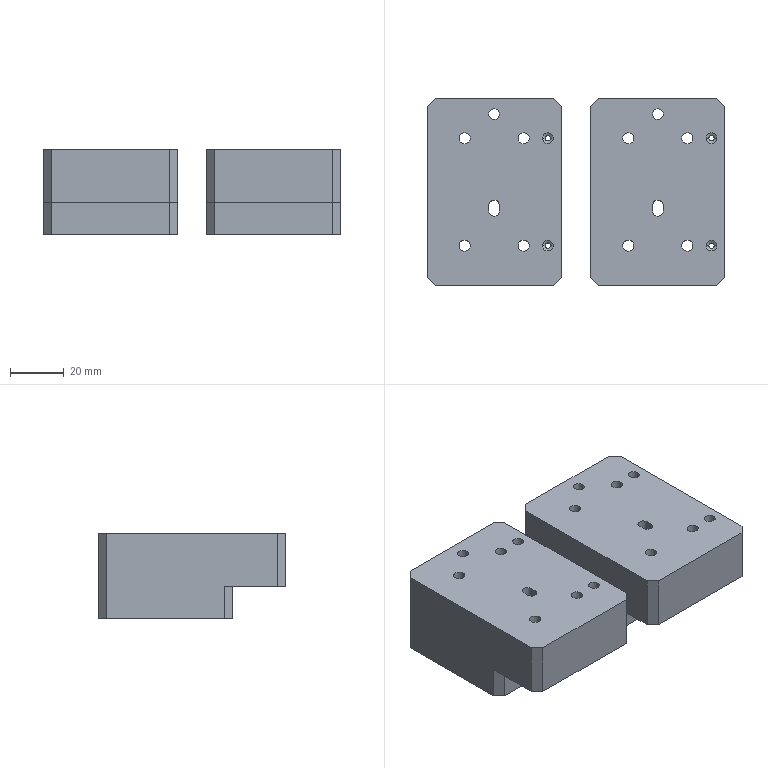NC program | NX | posted with a generic post | part box 111 x 70 x 32 mm
Lines 19 to 875 of 5357:
(ZLEVEL_PROFILE , TOOL : D10)
N36 T15 M6
N38 G54
N40 G17 G0 G90 X104.574 Y75.1 S9500 M3
N42 G43 Z30. H15
N44 Z1.5
N46 G94 G1 X108.554 Z1.291 F1000.
N48 X109.963 Y74.74 Z1.215
N50 X111.215 Y73.998 Z1.139
N52 X114.998 Y70.215 Z0.859
N54 X115.74 Y68.963 Z0.782
N56 X116.1 Y67.554 Z0.706
N58 Y35. Z-1.
N60 Y3. F3000.
N62 G2 X114.606 Y-0.606 R5.1
N64 G1 X111.606 Y-3.606
N66 G2 X108. Y-5.1 R5.1
N68 G1 X64.
N70 G2 X60.394 Y-3.606 R5.1
N72 G1 X57.394 Y-0.606
N74 G2 X55.9 Y3. R5.1
N76 G1 Y67.
N78 G2 X57.394 Y70.606 R5.1
N80 G1 X60.394 Y73.606
N82 G2 X64. Y75.1 R5.1
N84 G1 X108.
N86 G2 X111.606 Y73.606 R5.1
N88 G1 X114.606 Y70.606
N90 G2 X116.1 Y67. R5.1
N92 G1 Y35.
N94 Y3. Z-1.121
N96 X116.075 Y2.5 Z-1.123
N98 X116.002 Y2.005 Z-1.125
N100 X115.88 Y1.52 Z-1.126
N102 X115.712 Y1.048 Z-1.128
N104 X115.498 Y0.596 Z-1.13
N106 X115.24 Y0.167 Z-1.132
N108 X114.942 Y-0.235 Z-1.134
N110 X114.606 Y-0.606 Z-1.136
N112 X111.606 Y-3.606 Z-1.152
N114 X111.235 Y-3.942 Z-1.154
N116 X110.833 Y-4.24 Z-1.156
N118 X110.404 Y-4.498 Z-1.158
N120 X109.952 Y-4.712 Z-1.159
N122 X109.48 Y-4.88 Z-1.161
N124 X108.995 Y-5.002 Z-1.163
N126 X108.5 Y-5.075 Z-1.165
N128 X108. Y-5.1 Z-1.167
N130 X64. Z-1.333
N132 X63.5 Y-5.075 Z-1.335
N134 X63.005 Y-5.002 Z-1.337
N136 X62.52 Y-4.88 Z-1.339
N138 X62.048 Y-4.712 Z-1.341
N140 X61.596 Y-4.498 Z-1.342
N142 X61.167 Y-4.24 Z-1.344
N144 X60.765 Y-3.942 Z-1.346
N146 X60.394 Y-3.606 Z-1.348
N148 X57.394 Y-0.606 Z-1.364
N150 X57.058 Y-0.235 Z-1.366
N152 X56.76 Y0.167 Z-1.368
N154 X56.502 Y0.596 Z-1.37
N156 X56.288 Y1.048 Z-1.372
N158 X56.12 Y1.52 Z-1.374
N160 X55.998 Y2.005 Z-1.375
N162 X55.925 Y2.5 Z-1.377
N164 X55.9 Y3. Z-1.379
N166 Y67. Z-1.621
N168 X55.925 Y67.5 Z-1.623
N170 X55.998 Y67.995 Z-1.625
N172 X56.12 Y68.48 Z-1.626
N174 X56.288 Y68.952 Z-1.628
N176 X56.502 Y69.404 Z-1.63
N178 X56.76 Y69.833 Z-1.632
N180 X57.058 Y70.235 Z-1.634
N182 X57.394 Y70.606 Z-1.636
N184 X60.394 Y73.606 Z-1.652
N186 X60.765 Y73.942 Z-1.654
N188 X61.167 Y74.24 Z-1.656
N190 X61.596 Y74.498 Z-1.658
N192 X62.048 Y74.712 Z-1.659
N194 X62.52 Y74.88 Z-1.661
N196 X63.005 Y75.002 Z-1.663
N198 X63.5 Y75.075 Z-1.665
N200 X64. Y75.1 Z-1.667
N202 X108. Z-1.833
N204 X108.5 Y75.075 Z-1.835
N206 X108.995 Y75.002 Z-1.837
N208 X109.48 Y74.88 Z-1.839
N210 X109.952 Y74.712 Z-1.841
N212 X110.404 Y74.498 Z-1.842
N214 X110.833 Y74.24 Z-1.844
N216 X111.235 Y73.942 Z-1.846
N218 X111.606 Y73.606 Z-1.848
N220 X114.606 Y70.606 Z-1.864
N222 X114.942 Y70.235 Z-1.866
N224 X115.24 Y69.833 Z-1.868
N226 X115.498 Y69.404 Z-1.87
N228 X115.712 Y68.952 Z-1.872
N230 X115.88 Y68.48 Z-1.874
N232 X116.002 Y67.995 Z-1.875
N234 X116.075 Y67.5 Z-1.877
N236 X116.1 Y67. Z-1.879
N238 Y35. Z-2.
N240 Y3. Z-2.121
N242 X116.075 Y2.5 Z-2.123
N244 X116.002 Y2.005 Z-2.125
N246 X115.88 Y1.52 Z-2.126
N248 X115.712 Y1.048 Z-2.128
N250 X115.498 Y0.596 Z-2.13
N252 X115.24 Y0.167 Z-2.132
N254 X114.942 Y-0.235 Z-2.134
N256 X114.606 Y-0.606 Z-2.136
N258 X111.606 Y-3.606 Z-2.152
N260 X111.235 Y-3.942 Z-2.154
N262 X110.833 Y-4.24 Z-2.156
N264 X110.404 Y-4.498 Z-2.158
N266 X109.952 Y-4.712 Z-2.159
N268 X109.48 Y-4.88 Z-2.161
N270 X108.995 Y-5.002 Z-2.163
N272 X108.5 Y-5.075 Z-2.165
N274 X108. Y-5.1 Z-2.167
N276 X64. Z-2.333
N278 X63.5 Y-5.075 Z-2.335
N280 X63.005 Y-5.002 Z-2.337
N282 X62.52 Y-4.88 Z-2.339
N284 X62.048 Y-4.712 Z-2.341
N286 X61.596 Y-4.498 Z-2.342
N288 X61.167 Y-4.24 Z-2.344
N290 X60.765 Y-3.942 Z-2.346
N292 X60.394 Y-3.606 Z-2.348
N294 X57.394 Y-0.606 Z-2.364
N296 X57.058 Y-0.235 Z-2.366
N298 X56.76 Y0.167 Z-2.368
N300 X56.502 Y0.596 Z-2.37
N302 X56.288 Y1.048 Z-2.372
N304 X56.12 Y1.52 Z-2.374
N306 X55.998 Y2.005 Z-2.375
N308 X55.925 Y2.5 Z-2.377
N310 X55.9 Y3. Z-2.379
N312 Y67. Z-2.621
N314 X55.925 Y67.5 Z-2.623
N316 X55.998 Y67.995 Z-2.625
N318 X56.12 Y68.48 Z-2.626
N320 X56.288 Y68.952 Z-2.628
N322 X56.502 Y69.404 Z-2.63
N324 X56.76 Y69.833 Z-2.632
N326 X57.058 Y70.235 Z-2.634
N328 X57.394 Y70.606 Z-2.636
N330 X60.394 Y73.606 Z-2.652
N332 X60.765 Y73.942 Z-2.654
N334 X61.167 Y74.24 Z-2.656
N336 X61.596 Y74.498 Z-2.658
N338 X62.048 Y74.712 Z-2.659
N340 X62.52 Y74.88 Z-2.661
N342 X63.005 Y75.002 Z-2.663
N344 X63.5 Y75.075 Z-2.665
N346 X64. Y75.1 Z-2.667
N348 X108. Z-2.833
N350 X108.5 Y75.075 Z-2.835
N352 X108.995 Y75.002 Z-2.837
N354 X109.48 Y74.88 Z-2.839
N356 X109.952 Y74.712 Z-2.841
N358 X110.404 Y74.498 Z-2.842
N360 X110.833 Y74.24 Z-2.844
N362 X111.235 Y73.942 Z-2.846
N364 X111.606 Y73.606 Z-2.848
N366 X114.606 Y70.606 Z-2.864
N368 X114.942 Y70.235 Z-2.866
N370 X115.24 Y69.833 Z-2.868
N372 X115.498 Y69.404 Z-2.87
N374 X115.712 Y68.952 Z-2.872
N376 X115.88 Y68.48 Z-2.874
N378 X116.002 Y67.995 Z-2.875
N380 X116.075 Y67.5 Z-2.877
N382 X116.1 Y67. Z-2.879
N384 Y35. Z-3.
N386 Y3. Z-3.121
N388 X116.075 Y2.5 Z-3.123
N390 X116.002 Y2.005 Z-3.125
N392 X115.88 Y1.52 Z-3.126
N394 X115.712 Y1.048 Z-3.128
N396 X115.498 Y0.596 Z-3.13
N398 X115.24 Y0.167 Z-3.132
N400 X114.942 Y-0.235 Z-3.134
N402 X114.606 Y-0.606 Z-3.136
N404 X111.606 Y-3.606 Z-3.152
N406 X111.235 Y-3.942 Z-3.154
N408 X110.833 Y-4.24 Z-3.156
N410 X110.404 Y-4.498 Z-3.158
N412 X109.952 Y-4.712 Z-3.159
N414 X109.48 Y-4.88 Z-3.161
N416 X108.995 Y-5.002 Z-3.163
N418 X108.5 Y-5.075 Z-3.165
N420 X108. Y-5.1 Z-3.167
N422 X64. Z-3.333
N424 X63.5 Y-5.075 Z-3.335
N426 X63.005 Y-5.002 Z-3.337
N428 X62.52 Y-4.88 Z-3.339
N430 X62.048 Y-4.712 Z-3.341
N432 X61.596 Y-4.498 Z-3.342
N434 X61.167 Y-4.24 Z-3.344
N436 X60.765 Y-3.942 Z-3.346
N438 X60.394 Y-3.606 Z-3.348
N440 X57.394 Y-0.606 Z-3.364
N442 X57.058 Y-0.235 Z-3.366
N444 X56.76 Y0.167 Z-3.368
N446 X56.502 Y0.596 Z-3.37
N448 X56.288 Y1.048 Z-3.372
N450 X56.12 Y1.52 Z-3.374
N452 X55.998 Y2.005 Z-3.375
N454 X55.925 Y2.5 Z-3.377
N456 X55.9 Y3. Z-3.379
N458 Y67. Z-3.621
N460 X55.925 Y67.5 Z-3.623
N462 X55.998 Y67.995 Z-3.625
N464 X56.12 Y68.48 Z-3.626
N466 X56.288 Y68.952 Z-3.628
N468 X56.502 Y69.404 Z-3.63
N470 X56.76 Y69.833 Z-3.632
N472 X57.058 Y70.235 Z-3.634
N474 X57.394 Y70.606 Z-3.636
N476 X60.394 Y73.606 Z-3.652
N478 X60.765 Y73.942 Z-3.654
N480 X61.167 Y74.24 Z-3.656
N482 X61.596 Y74.498 Z-3.658
N484 X62.048 Y74.712 Z-3.659
N486 X62.52 Y74.88 Z-3.661
N488 X63.005 Y75.002 Z-3.663
N490 X63.5 Y75.075 Z-3.665
N492 X64. Y75.1 Z-3.667
N494 X108. Z-3.833
N496 X108.5 Y75.075 Z-3.835
N498 X108.995 Y75.002 Z-3.837
N500 X109.48 Y74.88 Z-3.839
N502 X109.952 Y74.712 Z-3.841
N504 X110.404 Y74.498 Z-3.842
N506 X110.833 Y74.24 Z-3.844
N508 X111.235 Y73.942 Z-3.846
N510 X111.606 Y73.606 Z-3.848
N512 X114.606 Y70.606 Z-3.864
N514 X114.942 Y70.235 Z-3.866
N516 X115.24 Y69.833 Z-3.868
N518 X115.498 Y69.404 Z-3.87
N520 X115.712 Y68.952 Z-3.872
N522 X115.88 Y68.48 Z-3.874
N524 X116.002 Y67.995 Z-3.875
N526 X116.075 Y67.5 Z-3.877
N528 X116.1 Y67. Z-3.879
N530 Y35. Z-4.
N532 Y3. Z-4.121
N534 X116.075 Y2.5 Z-4.123
N536 X116.002 Y2.005 Z-4.125
N538 X115.88 Y1.52 Z-4.126
N540 X115.712 Y1.048 Z-4.128
N542 X115.498 Y0.596 Z-4.13
N544 X115.24 Y0.167 Z-4.132
N546 X114.942 Y-0.235 Z-4.134
N548 X114.606 Y-0.606 Z-4.136
N550 X111.606 Y-3.606 Z-4.152
N552 X111.235 Y-3.942 Z-4.154
N554 X110.833 Y-4.24 Z-4.156
N556 X110.404 Y-4.498 Z-4.158
N558 X109.952 Y-4.712 Z-4.159
N560 X109.48 Y-4.88 Z-4.161
N562 X108.995 Y-5.002 Z-4.163
N564 X108.5 Y-5.075 Z-4.165
N566 X108. Y-5.1 Z-4.167
N568 X64. Z-4.333
N570 X63.5 Y-5.075 Z-4.335
N572 X63.005 Y-5.002 Z-4.337
N574 X62.52 Y-4.88 Z-4.339
N576 X62.048 Y-4.712 Z-4.341
N578 X61.596 Y-4.498 Z-4.342
N580 X61.167 Y-4.24 Z-4.344
N582 X60.765 Y-3.942 Z-4.346
N584 X60.394 Y-3.606 Z-4.348
N586 X57.394 Y-0.606 Z-4.364
N588 X57.058 Y-0.235 Z-4.366
N590 X56.76 Y0.167 Z-4.368
N592 X56.502 Y0.596 Z-4.37
N594 X56.288 Y1.048 Z-4.372
N596 X56.12 Y1.52 Z-4.374
N598 X55.998 Y2.005 Z-4.375
N600 X55.925 Y2.5 Z-4.377
N602 X55.9 Y3. Z-4.379
N604 Y67. Z-4.621
N606 X55.925 Y67.5 Z-4.623
N608 X55.998 Y67.995 Z-4.625
N610 X56.12 Y68.48 Z-4.626
N612 X56.288 Y68.952 Z-4.628
N614 X56.502 Y69.404 Z-4.63
N616 X56.76 Y69.833 Z-4.632
N618 X57.058 Y70.235 Z-4.634
N620 X57.394 Y70.606 Z-4.636
N622 X60.394 Y73.606 Z-4.652
N624 X60.765 Y73.942 Z-4.654
N626 X61.167 Y74.24 Z-4.656
N628 X61.596 Y74.498 Z-4.658
N630 X62.048 Y74.712 Z-4.659
N632 X62.52 Y74.88 Z-4.661
N634 X63.005 Y75.002 Z-4.663
N636 X63.5 Y75.075 Z-4.665
N638 X64. Y75.1 Z-4.667
N640 X108. Z-4.833
N642 X108.5 Y75.075 Z-4.835
N644 X108.995 Y75.002 Z-4.837
N646 X109.48 Y74.88 Z-4.839
N648 X109.952 Y74.712 Z-4.841
N650 X110.404 Y74.498 Z-4.842
N652 X110.833 Y74.24 Z-4.844
N654 X111.235 Y73.942 Z-4.846
N656 X111.606 Y73.606 Z-4.848
N658 X114.606 Y70.606 Z-4.864
N660 X114.942 Y70.235 Z-4.866
N662 X115.24 Y69.833 Z-4.868
N664 X115.498 Y69.404 Z-4.87
N666 X115.712 Y68.952 Z-4.872
N668 X115.88 Y68.48 Z-4.874
N670 X116.002 Y67.995 Z-4.875
N672 X116.075 Y67.5 Z-4.877
N674 X116.1 Y67. Z-4.879
N676 Y35. Z-5.
N678 Y3. Z-5.121
N680 X116.075 Y2.5 Z-5.123
N682 X116.002 Y2.005 Z-5.125
N684 X115.88 Y1.52 Z-5.126
N686 X115.712 Y1.048 Z-5.128
N688 X115.498 Y0.596 Z-5.13
N690 X115.24 Y0.167 Z-5.132
N692 X114.942 Y-0.235 Z-5.134
N694 X114.606 Y-0.606 Z-5.136
N696 X111.606 Y-3.606 Z-5.152
N698 X111.235 Y-3.942 Z-5.154
N700 X110.833 Y-4.24 Z-5.156
N702 X110.404 Y-4.498 Z-5.158
N704 X109.952 Y-4.712 Z-5.159
N706 X109.48 Y-4.88 Z-5.161
N708 X108.995 Y-5.002 Z-5.163
N710 X108.5 Y-5.075 Z-5.165
N712 X108. Y-5.1 Z-5.167
N714 X64. Z-5.333
N716 X63.5 Y-5.075 Z-5.335
N718 X63.005 Y-5.002 Z-5.337
N720 X62.52 Y-4.88 Z-5.339
N722 X62.048 Y-4.712 Z-5.341
N724 X61.596 Y-4.498 Z-5.342
N726 X61.167 Y-4.24 Z-5.344
N728 X60.765 Y-3.942 Z-5.346
N730 X60.394 Y-3.606 Z-5.348
N732 X57.394 Y-0.606 Z-5.364
N734 X57.058 Y-0.235 Z-5.366
N736 X56.76 Y0.167 Z-5.368
N738 X56.502 Y0.596 Z-5.37
N740 X56.288 Y1.048 Z-5.372
N742 X56.12 Y1.52 Z-5.374
N744 X55.998 Y2.005 Z-5.375
N746 X55.925 Y2.5 Z-5.377
N748 X55.9 Y3. Z-5.379
N750 Y67. Z-5.621
N752 X55.925 Y67.5 Z-5.623
N754 X55.998 Y67.995 Z-5.625
N756 X56.12 Y68.48 Z-5.626
N758 X56.288 Y68.952 Z-5.628
N760 X56.502 Y69.404 Z-5.63
N762 X56.76 Y69.833 Z-5.632
N764 X57.058 Y70.235 Z-5.634
N766 X57.394 Y70.606 Z-5.636
N768 X60.394 Y73.606 Z-5.652
N770 X60.765 Y73.942 Z-5.654
N772 X61.167 Y74.24 Z-5.656
N774 X61.596 Y74.498 Z-5.658
N776 X62.048 Y74.712 Z-5.659
N778 X62.52 Y74.88 Z-5.661
N780 X63.005 Y75.002 Z-5.663
N782 X63.5 Y75.075 Z-5.665
N784 X64. Y75.1 Z-5.667
N786 X108. Z-5.833
N788 X108.5 Y75.075 Z-5.835
N790 X108.995 Y75.002 Z-5.837
N792 X109.48 Y74.88 Z-5.839
N794 X109.952 Y74.712 Z-5.841
N796 X110.404 Y74.498 Z-5.842
N798 X110.833 Y74.24 Z-5.844
N800 X111.235 Y73.942 Z-5.846
N802 X111.606 Y73.606 Z-5.848
N804 X114.606 Y70.606 Z-5.864
N806 X114.942 Y70.235 Z-5.866
N808 X115.24 Y69.833 Z-5.868
N810 X115.498 Y69.404 Z-5.87
N812 X115.712 Y68.952 Z-5.872
N814 X115.88 Y68.48 Z-5.874
N816 X116.002 Y67.995 Z-5.875
N818 X116.075 Y67.5 Z-5.877
N820 X116.1 Y67. Z-5.879
N822 Y35. Z-6.
N824 Y3. Z-6.121
N826 X116.075 Y2.5 Z-6.123
N828 X116.002 Y2.005 Z-6.125
N830 X115.88 Y1.52 Z-6.126
N832 X115.712 Y1.048 Z-6.128
N834 X115.498 Y0.596 Z-6.13
N836 X115.24 Y0.167 Z-6.132
N838 X114.942 Y-0.235 Z-6.134
N840 X114.606 Y-0.606 Z-6.136
N842 X111.606 Y-3.606 Z-6.152
N844 X111.235 Y-3.942 Z-6.154
N846 X110.833 Y-4.24 Z-6.156
N848 X110.404 Y-4.498 Z-6.158
N850 X109.952 Y-4.712 Z-6.159
N852 X109.48 Y-4.88 Z-6.161
N854 X108.995 Y-5.002 Z-6.163
N856 X108.5 Y-5.075 Z-6.165
N858 X108. Y-5.1 Z-6.167
N860 X64. Z-6.333
N862 X63.5 Y-5.075 Z-6.335
N864 X63.005 Y-5.002 Z-6.337
N866 X62.52 Y-4.88 Z-6.339
N868 X62.048 Y-4.712 Z-6.341
N870 X61.596 Y-4.498 Z-6.342
N872 X61.167 Y-4.24 Z-6.344
N874 X60.765 Y-3.942 Z-6.346
N876 X60.394 Y-3.606 Z-6.348
N878 X57.394 Y-0.606 Z-6.364
N880 X57.058 Y-0.235 Z-6.366
N882 X56.76 Y0.167 Z-6.368
N884 X56.502 Y0.596 Z-6.37
N886 X56.288 Y1.048 Z-6.372
N888 X56.12 Y1.52 Z-6.374
N890 X55.998 Y2.005 Z-6.375
N892 X55.925 Y2.5 Z-6.377
N894 X55.9 Y3. Z-6.379
N896 Y67. Z-6.621
N898 X55.925 Y67.5 Z-6.623
N900 X55.998 Y67.995 Z-6.625
N902 X56.12 Y68.48 Z-6.626
N904 X56.288 Y68.952 Z-6.628
N906 X56.502 Y69.404 Z-6.63
N908 X56.76 Y69.833 Z-6.632
N910 X57.058 Y70.235 Z-6.634
N912 X57.394 Y70.606 Z-6.636
N914 X60.394 Y73.606 Z-6.652
N916 X60.765 Y73.942 Z-6.654
N918 X61.167 Y74.24 Z-6.656
N920 X61.596 Y74.498 Z-6.658
N922 X62.048 Y74.712 Z-6.659
N924 X62.52 Y74.88 Z-6.661
N926 X63.005 Y75.002 Z-6.663
N928 X63.5 Y75.075 Z-6.665
N930 X64. Y75.1 Z-6.667
N932 X108. Z-6.833
N934 X108.5 Y75.075 Z-6.835
N936 X108.995 Y75.002 Z-6.837
N938 X109.48 Y74.88 Z-6.839
N940 X109.952 Y74.712 Z-6.841
N942 X110.404 Y74.498 Z-6.842
N944 X110.833 Y74.24 Z-6.844
N946 X111.235 Y73.942 Z-6.846
N948 X111.606 Y73.606 Z-6.848
N950 X114.606 Y70.606 Z-6.864
N952 X114.942 Y70.235 Z-6.866
N954 X115.24 Y69.833 Z-6.868
N956 X115.498 Y69.404 Z-6.87
N958 X115.712 Y68.952 Z-6.872
N960 X115.88 Y68.48 Z-6.874
N962 X116.002 Y67.995 Z-6.875
N964 X116.075 Y67.5 Z-6.877
N966 X116.1 Y67. Z-6.879
N968 Y35. Z-7.
N970 Y3. Z-7.121
N972 X116.075 Y2.5 Z-7.123
N974 X116.002 Y2.005 Z-7.125
N976 X115.88 Y1.52 Z-7.126
N978 X115.712 Y1.048 Z-7.128
N980 X115.498 Y0.596 Z-7.13
N982 X115.24 Y0.167 Z-7.132
N984 X114.942 Y-0.235 Z-7.134
N986 X114.606 Y-0.606 Z-7.136
N988 X111.606 Y-3.606 Z-7.152
N990 X111.235 Y-3.942 Z-7.154
N992 X110.833 Y-4.24 Z-7.156
N994 X110.404 Y-4.498 Z-7.158
N996 X109.952 Y-4.712 Z-7.159
N998 X109.48 Y-4.88 Z-7.161
N1000 X108.995 Y-5.002 Z-7.163
N1002 X108.5 Y-5.075 Z-7.165
N1004 X108. Y-5.1 Z-7.167
N1006 X64. Z-7.333
N1008 X63.5 Y-5.075 Z-7.335
N1010 X63.005 Y-5.002 Z-7.337
N1012 X62.52 Y-4.88 Z-7.339
N1014 X62.048 Y-4.712 Z-7.341
N1016 X61.596 Y-4.498 Z-7.342
N1018 X61.167 Y-4.24 Z-7.344
N1020 X60.765 Y-3.942 Z-7.346
N1022 X60.394 Y-3.606 Z-7.348
N1024 X57.394 Y-0.606 Z-7.364
N1026 X57.058 Y-0.235 Z-7.366
N1028 X56.76 Y0.167 Z-7.368
N1030 X56.502 Y0.596 Z-7.37
N1032 X56.288 Y1.048 Z-7.372
N1034 X56.12 Y1.52 Z-7.374
N1036 X55.998 Y2.005 Z-7.375
N1038 X55.925 Y2.5 Z-7.377
N1040 X55.9 Y3. Z-7.379
N1042 Y67. Z-7.621
N1044 X55.925 Y67.5 Z-7.623
N1046 X55.998 Y67.995 Z-7.625
N1048 X56.12 Y68.48 Z-7.626
N1050 X56.288 Y68.952 Z-7.628
N1052 X56.502 Y69.404 Z-7.63
N1054 X56.76 Y69.833 Z-7.632
N1056 X57.058 Y70.235 Z-7.634
N1058 X57.394 Y70.606 Z-7.636
N1060 X60.394 Y73.606 Z-7.652
N1062 X60.765 Y73.942 Z-7.654
N1064 X61.167 Y74.24 Z-7.656
N1066 X61.596 Y74.498 Z-7.658
N1068 X62.048 Y74.712 Z-7.659
N1070 X62.52 Y74.88 Z-7.661
N1072 X63.005 Y75.002 Z-7.663
N1074 X63.5 Y75.075 Z-7.665
N1076 X64. Y75.1 Z-7.667
N1078 X108. Z-7.833
N1080 X108.5 Y75.075 Z-7.835
N1082 X108.995 Y75.002 Z-7.837
N1084 X109.48 Y74.88 Z-7.839
N1086 X109.952 Y74.712 Z-7.841
N1088 X110.404 Y74.498 Z-7.842
N1090 X110.833 Y74.24 Z-7.844
N1092 X111.235 Y73.942 Z-7.846
N1094 X111.606 Y73.606 Z-7.848
N1096 X114.606 Y70.606 Z-7.864
N1098 X114.942 Y70.235 Z-7.866
N1100 X115.24 Y69.833 Z-7.868
N1102 X115.498 Y69.404 Z-7.87
N1104 X115.712 Y68.952 Z-7.872
N1106 X115.88 Y68.48 Z-7.874
N1108 X116.002 Y67.995 Z-7.875
N1110 X116.075 Y67.5 Z-7.877
N1112 X116.1 Y67. Z-7.879
N1114 Y35. Z-8.
N1116 Y3. Z-8.121
N1118 X116.075 Y2.5 Z-8.123
N1120 X116.002 Y2.005 Z-8.125
N1122 X115.88 Y1.52 Z-8.126
N1124 X115.712 Y1.048 Z-8.128
N1126 X115.498 Y0.596 Z-8.13
N1128 X115.24 Y0.167 Z-8.132
N1130 X114.942 Y-0.235 Z-8.134
N1132 X114.606 Y-0.606 Z-8.136
N1134 X111.606 Y-3.606 Z-8.152
N1136 X111.235 Y-3.942 Z-8.154
N1138 X110.833 Y-4.24 Z-8.156
N1140 X110.404 Y-4.498 Z-8.158
N1142 X109.952 Y-4.712 Z-8.159
N1144 X109.48 Y-4.88 Z-8.161
N1146 X108.995 Y-5.002 Z-8.163
N1148 X108.5 Y-5.075 Z-8.165
N1150 X108. Y-5.1 Z-8.167
N1152 X64. Z-8.333
N1154 X63.5 Y-5.075 Z-8.335
N1156 X63.005 Y-5.002 Z-8.337
N1158 X62.52 Y-4.88 Z-8.339
N1160 X62.048 Y-4.712 Z-8.341
N1162 X61.596 Y-4.498 Z-8.342
N1164 X61.167 Y-4.24 Z-8.344
N1166 X60.765 Y-3.942 Z-8.346
N1168 X60.394 Y-3.606 Z-8.348
N1170 X57.394 Y-0.606 Z-8.364
N1172 X57.058 Y-0.235 Z-8.366
N1174 X56.76 Y0.167 Z-8.368
N1176 X56.502 Y0.596 Z-8.37
N1178 X56.288 Y1.048 Z-8.372
N1180 X56.12 Y1.52 Z-8.374
N1182 X55.998 Y2.005 Z-8.375
N1184 X55.925 Y2.5 Z-8.377
N1186 X55.9 Y3. Z-8.379
N1188 Y67. Z-8.621
N1190 X55.925 Y67.5 Z-8.623
N1192 X55.998 Y67.995 Z-8.625
N1194 X56.12 Y68.48 Z-8.626
N1196 X56.288 Y68.952 Z-8.628
N1198 X56.502 Y69.404 Z-8.63
N1200 X56.76 Y69.833 Z-8.632
N1202 X57.058 Y70.235 Z-8.634
N1204 X57.394 Y70.606 Z-8.636
N1206 X60.394 Y73.606 Z-8.652
N1208 X60.765 Y73.942 Z-8.654
N1210 X61.167 Y74.24 Z-8.656
N1212 X61.596 Y74.498 Z-8.658
N1214 X62.048 Y74.712 Z-8.659
N1216 X62.52 Y74.88 Z-8.661
N1218 X63.005 Y75.002 Z-8.663
N1220 X63.5 Y75.075 Z-8.665
N1222 X64. Y75.1 Z-8.667
N1224 X108. Z-8.833
N1226 X108.5 Y75.075 Z-8.835
N1228 X108.995 Y75.002 Z-8.837
N1230 X109.48 Y74.88 Z-8.839
N1232 X109.952 Y74.712 Z-8.841
N1234 X110.404 Y74.498 Z-8.842
N1236 X110.833 Y74.24 Z-8.844
N1238 X111.235 Y73.942 Z-8.846
N1240 X111.606 Y73.606 Z-8.848
N1242 X114.606 Y70.606 Z-8.864
N1244 X114.942 Y70.235 Z-8.866
N1246 X115.24 Y69.833 Z-8.868
N1248 X115.498 Y69.404 Z-8.87
N1250 X115.712 Y68.952 Z-8.872
N1252 X115.88 Y68.48 Z-8.874
N1254 X116.002 Y67.995 Z-8.875
N1256 X116.075 Y67.5 Z-8.877
N1258 X116.1 Y67. Z-8.879
N1260 Y35. Z-9.
N1262 Y3. Z-9.121
N1264 X116.075 Y2.5 Z-9.123
N1266 X116.002 Y2.005 Z-9.125
N1268 X115.88 Y1.52 Z-9.126
N1270 X115.712 Y1.048 Z-9.128
N1272 X115.498 Y0.596 Z-9.13
N1274 X115.24 Y0.167 Z-9.132
N1276 X114.942 Y-0.235 Z-9.134
N1278 X114.606 Y-0.606 Z-9.136
N1280 X111.606 Y-3.606 Z-9.152
N1282 X111.235 Y-3.942 Z-9.154
N1284 X110.833 Y-4.24 Z-9.156
N1286 X110.404 Y-4.498 Z-9.158
N1288 X109.952 Y-4.712 Z-9.159
N1290 X109.48 Y-4.88 Z-9.161
N1292 X108.995 Y-5.002 Z-9.163
N1294 X108.5 Y-5.075 Z-9.165
N1296 X108. Y-5.1 Z-9.167
N1298 X64. Z-9.333
N1300 X63.5 Y-5.075 Z-9.335
N1302 X63.005 Y-5.002 Z-9.337
N1304 X62.52 Y-4.88 Z-9.339
N1306 X62.048 Y-4.712 Z-9.341
N1308 X61.596 Y-4.498 Z-9.342
N1310 X61.167 Y-4.24 Z-9.344
N1312 X60.765 Y-3.942 Z-9.346
N1314 X60.394 Y-3.606 Z-9.348
N1316 X57.394 Y-0.606 Z-9.364
N1318 X57.058 Y-0.235 Z-9.366
N1320 X56.76 Y0.167 Z-9.368
N1322 X56.502 Y0.596 Z-9.37
N1324 X56.288 Y1.048 Z-9.372
N1326 X56.12 Y1.52 Z-9.374
N1328 X55.998 Y2.005 Z-9.375
N1330 X55.925 Y2.5 Z-9.377
N1332 X55.9 Y3. Z-9.379
N1334 Y67. Z-9.621
N1336 X55.925 Y67.5 Z-9.623
N1338 X55.998 Y67.995 Z-9.625
N1340 X56.12 Y68.48 Z-9.626
N1342 X56.288 Y68.952 Z-9.628
N1344 X56.502 Y69.404 Z-9.63
N1346 X56.76 Y69.833 Z-9.632
N1348 X57.058 Y70.235 Z-9.634
N1350 X57.394 Y70.606 Z-9.636
N1352 X60.394 Y73.606 Z-9.652
N1354 X60.765 Y73.942 Z-9.654
N1356 X61.167 Y74.24 Z-9.656
N1358 X61.596 Y74.498 Z-9.658
N1360 X62.048 Y74.712 Z-9.659
N1362 X62.52 Y74.88 Z-9.661
N1364 X63.005 Y75.002 Z-9.663
N1366 X63.5 Y75.075 Z-9.665
N1368 X64. Y75.1 Z-9.667
N1370 X108. Z-9.833
N1372 X108.5 Y75.075 Z-9.835
N1374 X108.995 Y75.002 Z-9.837
N1376 X109.48 Y74.88 Z-9.839
N1378 X109.952 Y74.712 Z-9.841
N1380 X110.404 Y74.498 Z-9.842
N1382 X110.833 Y74.24 Z-9.844
N1384 X111.235 Y73.942 Z-9.846
N1386 X111.606 Y73.606 Z-9.848
N1388 X114.606 Y70.606 Z-9.864
N1390 X114.942 Y70.235 Z-9.866
N1392 X115.24 Y69.833 Z-9.868
N1394 X115.498 Y69.404 Z-9.87
N1396 X115.712 Y68.952 Z-9.872
N1398 X115.88 Y68.48 Z-9.874
N1400 X116.002 Y67.995 Z-9.875
N1402 X116.075 Y67.5 Z-9.877
N1404 X116.1 Y67. Z-9.879
N1406 Y35. Z-10.
N1408 Y3. Z-10.121
N1410 X116.075 Y2.5 Z-10.123
N1412 X116.002 Y2.005 Z-10.125
N1414 X115.88 Y1.52 Z-10.126
N1416 X115.712 Y1.048 Z-10.128
N1418 X115.498 Y0.596 Z-10.13
N1420 X115.24 Y0.167 Z-10.132
N1422 X114.942 Y-0.235 Z-10.134
N1424 X114.606 Y-0.606 Z-10.136
N1426 X111.606 Y-3.606 Z-10.152
N1428 X111.235 Y-3.942 Z-10.154
N1430 X110.833 Y-4.24 Z-10.156
N1432 X110.404 Y-4.498 Z-10.158
N1434 X109.952 Y-4.712 Z-10.159
N1436 X109.48 Y-4.88 Z-10.161
N1438 X108.995 Y-5.002 Z-10.163
N1440 X108.5 Y-5.075 Z-10.165
N1442 X108. Y-5.1 Z-10.167
N1444 X64. Z-10.333
N1446 X63.5 Y-5.075 Z-10.335
N1448 X63.005 Y-5.002 Z-10.337
N1450 X62.52 Y-4.88 Z-10.339
N1452 X62.048 Y-4.712 Z-10.341
N1454 X61.596 Y-4.498 Z-10.342
N1456 X61.167 Y-4.24 Z-10.344
N1458 X60.765 Y-3.942 Z-10.346
N1460 X60.394 Y-3.606 Z-10.348
N1462 X57.394 Y-0.606 Z-10.364
N1464 X57.058 Y-0.235 Z-10.366
N1466 X56.76 Y0.167 Z-10.368
N1468 X56.502 Y0.596 Z-10.37
N1470 X56.288 Y1.048 Z-10.372
N1472 X56.12 Y1.52 Z-10.374
N1474 X55.998 Y2.005 Z-10.375
N1476 X55.925 Y2.5 Z-10.377
N1478 X55.9 Y3. Z-10.379
N1480 Y67. Z-10.621
N1482 X55.925 Y67.5 Z-10.623
N1484 X55.998 Y67.995 Z-10.625
N1486 X56.12 Y68.48 Z-10.626
N1488 X56.288 Y68.952 Z-10.628
N1490 X56.502 Y69.404 Z-10.63
N1492 X56.76 Y69.833 Z-10.632
N1494 X57.058 Y70.235 Z-10.634
N1496 X57.394 Y70.606 Z-10.636
N1498 X60.394 Y73.606 Z-10.652
N1500 X60.765 Y73.942 Z-10.654
N1502 X61.167 Y74.24 Z-10.656
N1504 X61.596 Y74.498 Z-10.658
N1506 X62.048 Y74.712 Z-10.659
N1508 X62.52 Y74.88 Z-10.661
N1510 X63.005 Y75.002 Z-10.663
N1512 X63.5 Y75.075 Z-10.665
N1514 X64. Y75.1 Z-10.667
N1516 X108. Z-10.833
N1518 X108.5 Y75.075 Z-10.835
N1520 X108.995 Y75.002 Z-10.837
N1522 X109.48 Y74.88 Z-10.839
N1524 X109.952 Y74.712 Z-10.841
N1526 X110.404 Y74.498 Z-10.842
N1528 X110.833 Y74.24 Z-10.844
N1530 X111.235 Y73.942 Z-10.846
N1532 X111.606 Y73.606 Z-10.848
N1534 X114.606 Y70.606 Z-10.864
N1536 X114.942 Y70.235 Z-10.866
N1538 X115.24 Y69.833 Z-10.868
N1540 X115.498 Y69.404 Z-10.87
N1542 X115.712 Y68.952 Z-10.872
N1544 X115.88 Y68.48 Z-10.874
N1546 X116.002 Y67.995 Z-10.875
N1548 X116.075 Y67.5 Z-10.877
N1550 X116.1 Y67. Z-10.879
N1552 Y35. Z-11.
N1554 Y3. Z-11.121
N1556 X116.075 Y2.5 Z-11.123
N1558 X116.002 Y2.005 Z-11.125
N1560 X115.88 Y1.52 Z-11.126
N1562 X115.712 Y1.048 Z-11.128
N1564 X115.498 Y0.596 Z-11.13
N1566 X115.24 Y0.167 Z-11.132
N1568 X114.942 Y-0.235 Z-11.134
N1570 X114.606 Y-0.606 Z-11.136
N1572 X111.606 Y-3.606 Z-11.152
N1574 X111.235 Y-3.942 Z-11.154
N1576 X110.833 Y-4.24 Z-11.156
N1578 X110.404 Y-4.498 Z-11.158
N1580 X109.952 Y-4.712 Z-11.159
N1582 X109.48 Y-4.88 Z-11.161
N1584 X108.995 Y-5.002 Z-11.163
N1586 X108.5 Y-5.075 Z-11.165
N1588 X108. Y-5.1 Z-11.167
N1590 X64. Z-11.333
N1592 X63.5 Y-5.075 Z-11.335
N1594 X63.005 Y-5.002 Z-11.337
N1596 X62.52 Y-4.88 Z-11.339
N1598 X62.048 Y-4.712 Z-11.341
N1600 X61.596 Y-4.498 Z-11.342
N1602 X61.167 Y-4.24 Z-11.344
N1604 X60.765 Y-3.942 Z-11.346
N1606 X60.394 Y-3.606 Z-11.348
N1608 X57.394 Y-0.606 Z-11.364
N1610 X57.058 Y-0.235 Z-11.366
N1612 X56.76 Y0.167 Z-11.368
N1614 X56.502 Y0.596 Z-11.37
N1616 X56.288 Y1.048 Z-11.372
N1618 X56.12 Y1.52 Z-11.374
N1620 X55.998 Y2.005 Z-11.375
N1622 X55.925 Y2.5 Z-11.377
N1624 X55.9 Y3. Z-11.379
N1626 Y67. Z-11.621
N1628 X55.925 Y67.5 Z-11.623
N1630 X55.998 Y67.995 Z-11.625
N1632 X56.12 Y68.48 Z-11.626
N1634 X56.288 Y68.952 Z-11.628
N1636 X56.502 Y69.404 Z-11.63
N1638 X56.76 Y69.833 Z-11.632
N1640 X57.058 Y70.235 Z-11.634
N1642 X57.394 Y70.606 Z-11.636
N1644 X60.394 Y73.606 Z-11.652
N1646 X60.765 Y73.942 Z-11.654
N1648 X61.167 Y74.24 Z-11.656
N1650 X61.596 Y74.498 Z-11.658
N1652 X62.048 Y74.712 Z-11.659
N1654 X62.52 Y74.88 Z-11.661
N1656 X63.005 Y75.002 Z-11.663
N1658 X63.5 Y75.075 Z-11.665
N1660 X64. Y75.1 Z-11.667
N1662 X108. Z-11.833
N1664 X108.5 Y75.075 Z-11.835
N1666 X108.995 Y75.002 Z-11.837
N1668 X109.48 Y74.88 Z-11.839
N1670 X109.952 Y74.712 Z-11.841
N1672 X110.404 Y74.498 Z-11.842
N1674 X110.833 Y74.24 Z-11.844
N1676 X111.235 Y73.942 Z-11.846
N1678 X111.606 Y73.606 Z-11.848
N1680 X114.606 Y70.606 Z-11.864
N1682 X114.942 Y70.235 Z-11.866
N1684 X115.24 Y69.833 Z-11.868
N1686 X115.498 Y69.404 Z-11.87
N1688 X115.712 Y68.952 Z-11.872
N1690 X115.88 Y68.48 Z-11.874
N1692 X116.002 Y67.995 Z-11.875
N1694 X116.075 Y67.5 Z-11.877
N1696 X116.1 Y67. Z-11.879
N1698 Y35. Z-12.
N1700 Y3. Z-12.121
N1702 X116.075 Y2.5 Z-12.123
N1704 X116.002 Y2.005 Z-12.125
N1706 X115.88 Y1.52 Z-12.126
N1708 X115.712 Y1.048 Z-12.128
N1710 X115.498 Y0.596 Z-12.13
N1712 X115.24 Y0.167 Z-12.132
N1714 X114.942 Y-0.235 Z-12.134
N1716 X114.606 Y-0.606 Z-12.136
N1718 X111.606 Y-3.606 Z-12.152
N1720 X111.235 Y-3.942 Z-12.154
N1722 X110.833 Y-4.24 Z-12.156
N1724 X110.404 Y-4.498 Z-12.158
N1726 X109.952 Y-4.712 Z-12.159
N1728 X109.48 Y-4.88 Z-12.161
N1730 X108.995 Y-5.002 Z-12.163
N1732 X108.5 Y-5.075 Z-12.165
N1734 X108. Y-5.1 Z-12.167
N1736 X64. Z-12.333
N1738 X63.5 Y-5.075 Z-12.335
N1740 X63.005 Y-5.002 Z-12.337
N1742 X62.52 Y-4.88 Z-12.339